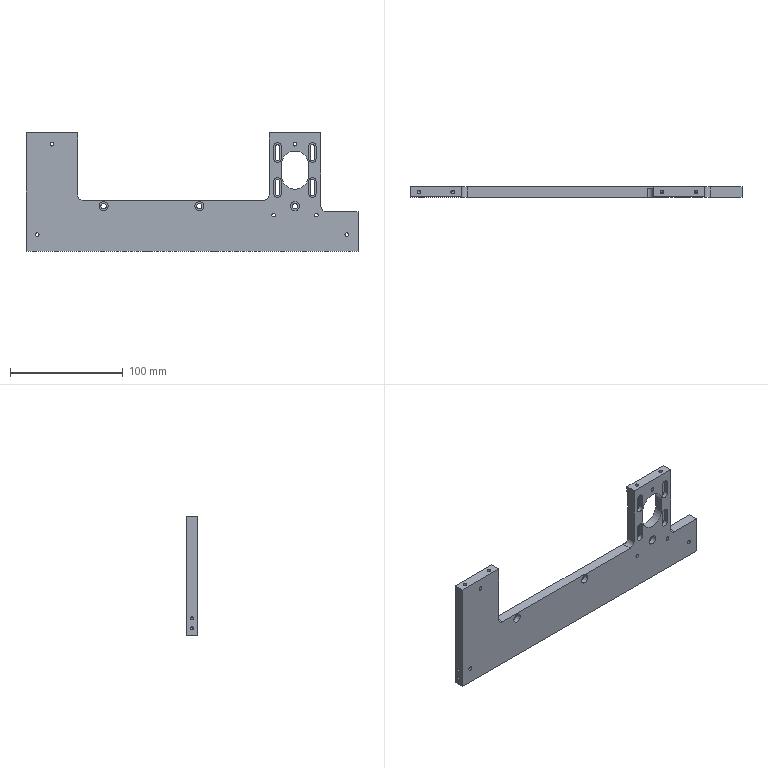Part | 1 solid | 127 faces | box 295 x 9 x 105 mm | volume 153354 mm3 | cylinder 62 | plane 40 | cone 25 | commonest cylinder face diameters 2.5 x25 3.3 x10 3.4 x8 6.5 x8 4.8 x3 8 x3